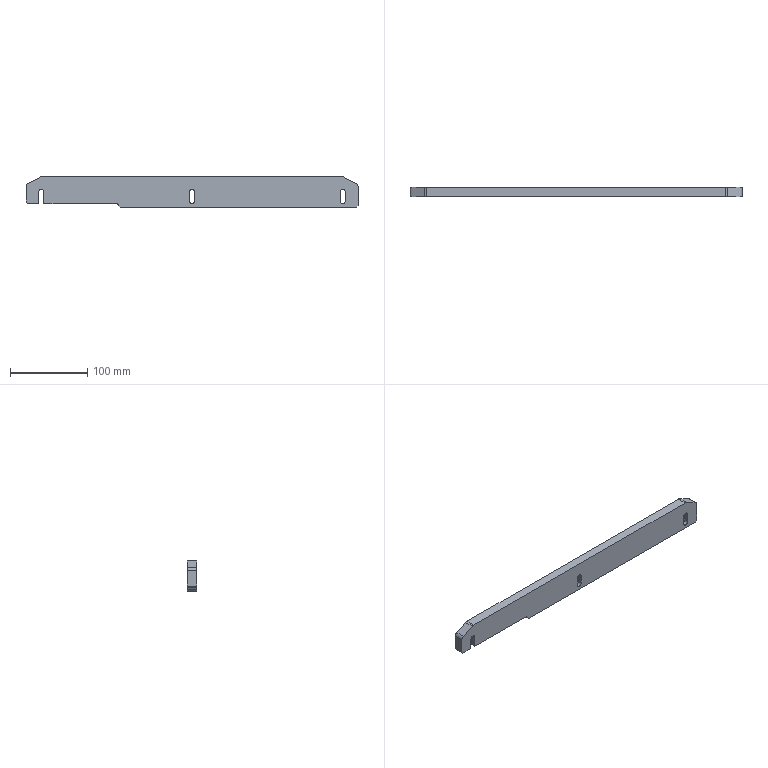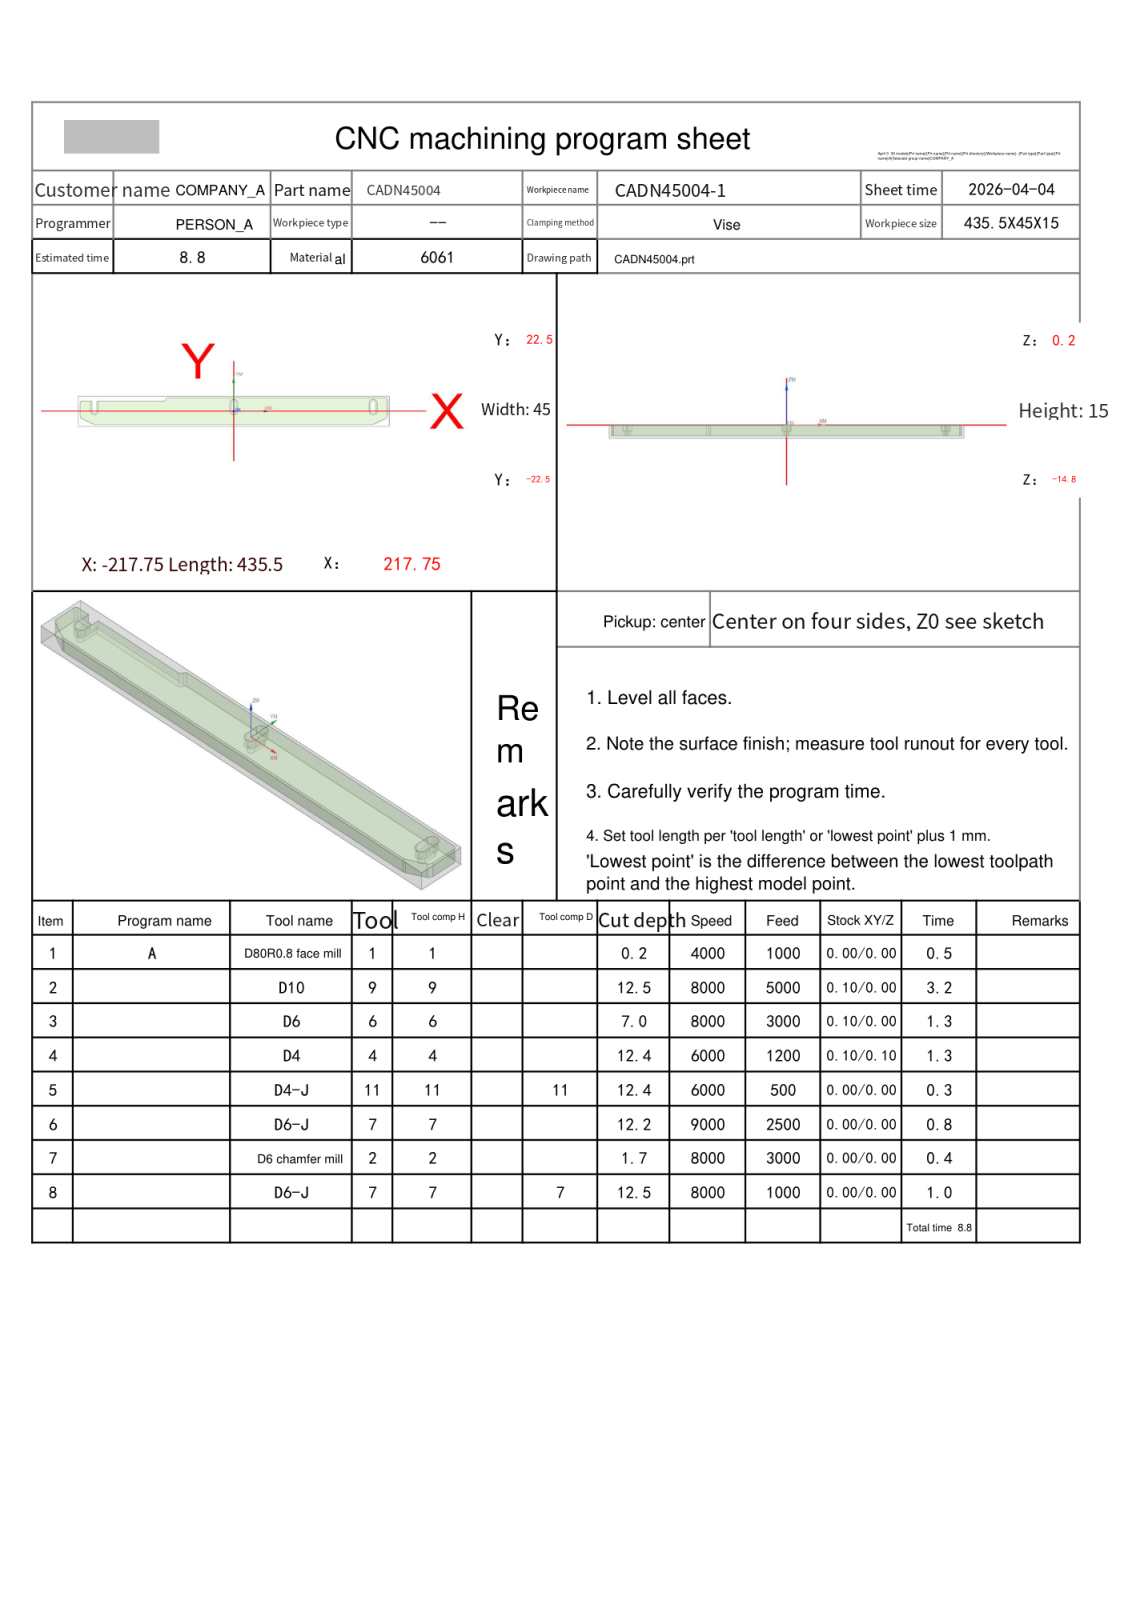NC program | NX | posted by the shop | part box 430.5 x 12 x 40 mm
Lines 3270 to 3420 of 3420:
N7 T02 M06
(D6 chamfer mill  D=6. R=0. H=02 ce=0.00 di=0.00)
G00 G90 G54 X.25 Y-22.128 M03 S8000
G43 H02 Z20.
M08
Z2.099
G01 Z-1.5 F3000.
G03 X.33 Y-21.828 I-.52 J.3
X.03 Y-21.308 I-.6 J0.0
G01 X0.0 Y-21.3
X-194.07
G02 X-196.887 Y-20.635 I0.0 J6.3
G01 X-213.067 Y-12.545
G02 X-216.55 Y-6.91 I2.817 J5.635
G01 Y13.
X-216.525 Y13.254
X-216.451 Y13.497
X-216.331 Y13.722
X-216.169 Y13.919
X-214.169 Y15.919
X-213.972 Y16.081
X-213.747 Y16.201
X-213.504 Y16.275
X-213.25 Y16.3
X-200.75
G02 X-199.45 Y15. I0.0 J-1.3
G01 Y0.0
G03 X-195.25 Y-4.2 I4.2 J0.0
X-191.05 Y0.0 I0.0 J4.2
G01 Y15.
G02 X-189.75 Y16.3 I1.3 J0.0
G01 X-98.25
G03 X-96.55 Y18. I0.0 J1.7
G01 X-96.525 Y18.254
X-96.451 Y18.497
X-96.331 Y18.722
X-96.169 Y18.919
X-94.169 Y20.919
X-93.972 Y21.081
X-93.747 Y21.201
X-93.504 Y21.275
X-93.25 Y21.3
X213.25
X213.504 Y21.275
X213.747 Y21.201
X213.972 Y21.081
X214.169 Y20.919
X216.169 Y18.919
X216.331 Y18.722
X216.451 Y18.497
X216.525 Y18.254
X216.55 Y18.
Y-6.91
G02 X213.067 Y-12.545 I-6.3 J0.0
G01 X196.887 Y-20.635
G02 X194.07 Y-21.3 I-2.817 J5.635
G01 X0.0
X-.03 Y-21.308
G03 X-.33 Y-21.828 I.3 J-.52
X-.25 Y-22.128 I.6 J0.0
G01 Z2.099
G00 Z20.
X-3.372 Y6.25
Z2.099
G01 Z-1.5
G03 X-3.672 Y6.33 I-.3 J-.52
X-4.192 Y6.03 I0.0 J-.6
G01 X-4.2 Y6.
Y0.0
G03 X0.0 Y-4.2 I4.2 J0.0
X4.2 Y0.0 I0.0 J4.2
G01 Y12.
G03 X0.0 Y16.2 I-4.2 J0.0
X-4.2 Y12. I0.0 J-4.2
G01 Y6.
X-4.192 Y5.97
G03 X-3.672 Y5.67 I.52 J.3
X-3.372 Y5.75 I0.0 J.6
G01 Z2.099
G00 Z20.
X191.878 Y6.25
Z2.099
G01 Z-1.5
G03 X191.578 Y6.33 I-.3 J-.52
X191.058 Y6.03 I0.0 J-.6
G01 X191.05 Y6.
Y0.0
G03 X195.25 Y-4.2 I4.2 J0.0
X199.45 Y0.0 I0.0 J4.2
G01 Y12.
G03 X195.25 Y16.2 I-4.2 J0.0
X191.05 Y12. I0.0 J-4.2
G01 Y6.
X191.058 Y5.97
G03 X191.578 Y5.67 I.52 J.3
X191.878 Y5.75 I0.0 J.6
G01 Z2.099
G00 Z20.
G91 G28 Z0.0
M05
M09
G91 G28 Z0.0
M01
N8 T07 M06
(D6-J  D=6. R=0. H=07 ce=0.00 di=0.00)
G00 G90 G54 X195.079 Y-24.144 M03 S8000
G43 H07 Z20.
M08
Z-11.8
G01 Z-12.3 F1000.
G41 D07
X195.068 Y-23.944
G03 X194.07 Y-23. I-.998 J-.056
G01 X-194.07
G02 X-197.647 Y-22.155 I0.0 J8.
G01 X-213.828 Y-14.065
G02 X-218.25 Y-6.91 I3.578 J7.155
G01 Y13.
G02 X-217.371 Y15.121 I3. J0.0
G01 X-215.371 Y17.121
G02 X-213.25 Y18. I2.121 J-2.121
G01 X-198.55
G02 X-195.55 Y15. I0.0 J-3.
G01 Y0.0
G03 X-195.25 Y-.3 I.3 J0.0
X-194.95 Y0.0 I0.0 J.3
G01 Y15.
G02 X-191.95 Y18. I3. J0.0
G01 X-98.25
G02 X-97.371 Y20.121 I3. J0.0
G01 X-95.371 Y22.121
G02 X-93.25 Y23. I2.121 J-2.121
G01 X213.25
G02 X215.371 Y22.121 I0.0 J-3.
G01 X217.371 Y20.121
G02 X218.25 Y18. I-2.121 J-2.121
G01 Y-6.91
G02 X213.828 Y-14.065 I-8. J0.0
G01 X197.647 Y-22.155
G02 X194.07 Y-23. I-3.578 J7.155
G01 X193.57
G03 X192.57 Y-24. I0.0 J-1.
G01 G40 Y-24.2
Z-11.8
G00 Z20.
M05
M09
G91 G28 Z0.0
G91 G28 Y0.0
M30
%